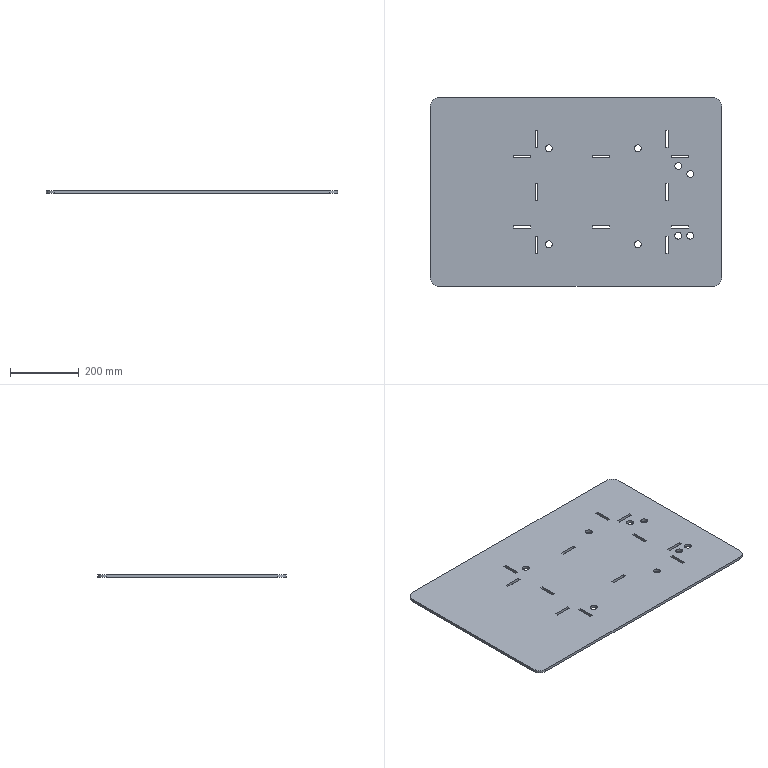Part | SolidWorks | features FlatPattern 1, SMBaseFlange 1, SheetMetal 1 | 1 solid | 74 faces | box 850 x 550 x 8 mm | volume 3677202 mm3 | plane 54 | cylinder 20 | commonest cylinder face diameters 20 x16 50 x4